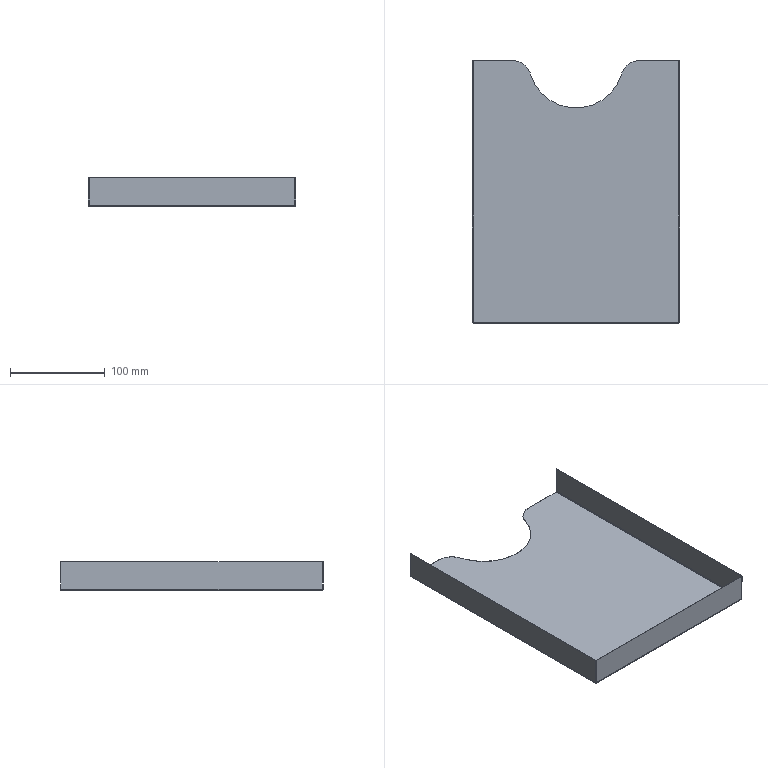Part | SolidWorks | features MirrorStock 1 | 1 solid | 34 faces | box 219 x 277 x 30 mm | volume 39482 mm3 | plane 21 | cylinder 9 | spline 4 | commonest cylinder face diameters 1.473 x3 2.473 x3 40 x2 100 x1
STEP:
#1=CARTESIAN_POINT('',(-67.082,138.5,0.));
#2=VERTEX_POINT('',#1);
#3=CARTESIAN_POINT('',(-108.263,138.5,0.));
#4=VERTEX_POINT('',#3);
#5=CARTESIAN_POINT('',(-109.5,138.5,0.));
#6=DIRECTION('',(-1.,0.,0.));
#7=VECTOR('',#6,1000.);
#8=LINE('',#5,#7);
#9=EDGE_CURVE('',#2,#4,#8,.T.);
#10=ORIENTED_EDGE('',*,*,#9,.T.);
#11=CARTESIAN_POINT('',(-108.263,138.5,0.5));
#12=VERTEX_POINT('',#11);
#13=CARTESIAN_POINT('',(-108.263,138.5,0.5));
#14=DIRECTION('',(0.,0.,-1.));
#15=VECTOR('',#14,1000.);
#16=LINE('',#13,#15);
#17=EDGE_CURVE('',#12,#4,#16,.T.);
#18=ORIENTED_EDGE('',*,*,#17,.F.);
#19=CARTESIAN_POINT('',(-67.082,138.5,0.5));
#20=VERTEX_POINT('',#19);
#21=CARTESIAN_POINT('',(-109.5,138.5,0.5));
#22=DIRECTION('',(-1.,0.,0.));
#23=VECTOR('',#22,1000.);
#24=LINE('',#21,#23);
#25=EDGE_CURVE('',#20,#12,#24,.T.);
#26=ORIENTED_EDGE('',*,*,#25,.F.);
#27=CARTESIAN_POINT('',(-67.082,138.5,0.5));
#28=DIRECTION('',(0.,0.,1.));
#29=VECTOR('',#28,1000.);
#30=LINE('',#27,#29);
#31=EDGE_CURVE('',#2,#20,#30,.T.);
#32=ORIENTED_EDGE('',*,*,#31,.F.);
#33=EDGE_LOOP('',(#10,#18,#26,#32));
#34=FACE_OUTER_BOUND('',#33,.T.);
#35=CARTESIAN_POINT('',(-109.5,138.5,0.5));
#36=DIRECTION('',(0.,1.,0.));
#37=DIRECTION('',(0.,0.,-1.));
#38=AXIS2_PLACEMENT_3D('',#35,#36,#37);
#39=PLANE('',#38);
#40=ADVANCED_FACE('',(#34),#39,.T.);
#41=CARTESIAN_POINT('',(-47.916,124.214,0.5));
#42=VERTEX_POINT('',#41);
#43=CARTESIAN_POINT('',(47.916,124.214,0.5));
#44=VERTEX_POINT('',#43);
#45=CARTESIAN_POINT('',(0.,138.5,0.5));
#46=DIRECTION('',(0.,0.,1.));
#47=DIRECTION('',(0.,-1.,0.));
#48=AXIS2_PLACEMENT_3D('',#45,#46,#47);
#49=CIRCLE('',#48,50.);
#50=EDGE_CURVE('',#42,#44,#49,.T.);
#51=ORIENTED_EDGE('',*,*,#50,.F.);
#52=CARTESIAN_POINT('',(-67.082,118.5,0.5));
#53=DIRECTION('',(0.,0.,-1.));
#54=DIRECTION('',(0.,-1.,0.));
#55=AXIS2_PLACEMENT_3D('',#52,#53,#54);
#56=CIRCLE('',#55,20.);
#57=EDGE_CURVE('',#20,#42,#56,.T.);
#58=ORIENTED_EDGE('',*,*,#57,.F.);
#59=ORIENTED_EDGE('',*,*,#25,.T.);
#60=CARTESIAN_POINT('',(-108.263,-137.263,0.5));
#61=VERTEX_POINT('',#60);
#62=CARTESIAN_POINT('',(-108.263,138.5,0.5));
#63=DIRECTION('',(0.,-1.,0.));
#64=VECTOR('',#63,1000.);
#65=LINE('',#62,#64);
#66=EDGE_CURVE('',#12,#61,#65,.T.);
#67=ORIENTED_EDGE('',*,*,#66,.T.);
#68=CARTESIAN_POINT('',(108.263,-137.263,0.5));
#69=VERTEX_POINT('',#68);
#70=CARTESIAN_POINT('',(-108.293,-137.263,0.5));
#71=DIRECTION('',(1.,0.,0.));
#72=VECTOR('',#71,1000.);
#73=LINE('',#70,#72);
#74=EDGE_CURVE('',#61,#69,#73,.T.);
#75=ORIENTED_EDGE('',*,*,#74,.T.);
#76=CARTESIAN_POINT('',(108.263,138.5,0.5));
#77=VERTEX_POINT('',#76);
#78=CARTESIAN_POINT('',(108.263,-137.293,0.5));
#79=DIRECTION('',(0.,1.,0.));
#80=VECTOR('',#79,1000.);
#81=LINE('',#78,#80);
#82=EDGE_CURVE('',#69,#77,#81,.T.);
#83=ORIENTED_EDGE('',*,*,#82,.T.);
#84=CARTESIAN_POINT('',(67.082,138.5,0.5));
#85=VERTEX_POINT('',#84);
#86=CARTESIAN_POINT('',(-109.5,138.5,0.5));
#87=DIRECTION('',(-1.,0.,0.));
#88=VECTOR('',#87,1000.);
#89=LINE('',#86,#88);
#90=EDGE_CURVE('',#77,#85,#89,.T.);
#91=ORIENTED_EDGE('',*,*,#90,.T.);
#92=CARTESIAN_POINT('',(67.082,118.5,0.5));
#93=DIRECTION('',(0.,0.,-1.));
#94=DIRECTION('',(0.,-1.,0.));
#95=AXIS2_PLACEMENT_3D('',#92,#93,#94);
#96=CIRCLE('',#95,20.);
#97=EDGE_CURVE('',#44,#85,#96,.T.);
#98=ORIENTED_EDGE('',*,*,#97,.F.);
#99=EDGE_LOOP('',(#51,#58,#59,#67,#75,#83,#91,#98));
#100=FACE_OUTER_BOUND('',#99,.T.);
#101=CARTESIAN_POINT('',(0.,0.,0.5));
#102=DIRECTION('',(0.,0.,-1.));
#103=DIRECTION('',(1.,0.,0.));
#104=AXIS2_PLACEMENT_3D('',#101,#102,#103);
#105=PLANE('',#104);
#106=ADVANCED_FACE('',(#100),#105,.F.);
#107=CARTESIAN_POINT('',(108.263,138.5,0.));
#108=VERTEX_POINT('',#107);
#109=CARTESIAN_POINT('',(67.082,138.5,0.));
#110=VERTEX_POINT('',#109);
#111=CARTESIAN_POINT('',(-109.5,138.5,0.));
#112=DIRECTION('',(-1.,0.,0.));
#113=VECTOR('',#112,1000.);
#114=LINE('',#111,#113);
#115=EDGE_CURVE('',#108,#110,#114,.T.);
#116=ORIENTED_EDGE('',*,*,#115,.F.);
#117=CARTESIAN_POINT('',(108.263,-137.263,0.));
#118=VERTEX_POINT('',#117);
#119=CARTESIAN_POINT('',(108.263,-137.293,0.));
#120=DIRECTION('',(0.,1.,0.));
#121=VECTOR('',#120,1000.);
#122=LINE('',#119,#121);
#123=EDGE_CURVE('',#118,#108,#122,.T.);
#124=ORIENTED_EDGE('',*,*,#123,.F.);
#125=CARTESIAN_POINT('',(-108.263,-137.263,0.));
#126=VERTEX_POINT('',#125);
#127=CARTESIAN_POINT('',(-108.293,-137.263,0.));
#128=DIRECTION('',(1.,0.,0.));
#129=VECTOR('',#128,1000.);
#130=LINE('',#127,#129);
#131=EDGE_CURVE('',#126,#118,#130,.T.);
#132=ORIENTED_EDGE('',*,*,#131,.F.);
#133=CARTESIAN_POINT('',(-108.263,138.5,0.));
#134=DIRECTION('',(0.,-1.,0.));
#135=VECTOR('',#134,1000.);
#136=LINE('',#133,#135);
#137=EDGE_CURVE('',#4,#126,#136,.T.);
#138=ORIENTED_EDGE('',*,*,#137,.F.);
#139=ORIENTED_EDGE('',*,*,#9,.F.);
#140=CARTESIAN_POINT('',(-47.916,124.214,0.));
#141=VERTEX_POINT('',#140);
#142=CARTESIAN_POINT('',(-67.082,118.5,0.));
#143=DIRECTION('',(0.,0.,1.));
#144=DIRECTION('',(0.,-1.,0.));
#145=AXIS2_PLACEMENT_3D('',#142,#143,#144);
#146=CIRCLE('',#145,20.);
#147=EDGE_CURVE('',#141,#2,#146,.T.);
#148=ORIENTED_EDGE('',*,*,#147,.F.);
#149=CARTESIAN_POINT('',(47.916,124.214,0.));
#150=VERTEX_POINT('',#149);
#151=CARTESIAN_POINT('',(0.,138.5,0.));
#152=DIRECTION('',(0.,0.,1.));
#153=DIRECTION('',(1.,0.,0.));
#154=AXIS2_PLACEMENT_3D('',#151,#152,#153);
#155=CIRCLE('',#154,50.);
#156=EDGE_CURVE('',#141,#150,#155,.T.);
#157=ORIENTED_EDGE('',*,*,#156,.T.);
#158=CARTESIAN_POINT('',(67.082,118.5,0.));
#159=DIRECTION('',(0.,0.,1.));
#160=DIRECTION('',(0.,-1.,0.));
#161=AXIS2_PLACEMENT_3D('',#158,#159,#160);
#162=CIRCLE('',#161,20.);
#163=EDGE_CURVE('',#110,#150,#162,.T.);
#164=ORIENTED_EDGE('',*,*,#163,.F.);
#165=EDGE_LOOP('',(#116,#124,#132,#138,#139,#148,#157,#164));
#166=FACE_OUTER_BOUND('',#165,.T.);
#167=CARTESIAN_POINT('',(0.,0.,0.));
#168=DIRECTION('',(0.,0.,-1.));
#169=DIRECTION('',(1.,0.,0.));
#170=AXIS2_PLACEMENT_3D('',#167,#168,#169);
#171=PLANE('',#170);
#172=ADVANCED_FACE('',(#166),#171,.T.);
#173=ORIENTED_EDGE('',*,*,#90,.F.);
#174=CARTESIAN_POINT('',(108.263,138.5,0.5));
#175=DIRECTION('',(0.,0.,-1.));
#176=VECTOR('',#175,1000.);
#177=LINE('',#174,#176);
#178=EDGE_CURVE('',#77,#108,#177,.T.);
#179=ORIENTED_EDGE('',*,*,#178,.T.);
#180=ORIENTED_EDGE('',*,*,#115,.T.);
#181=CARTESIAN_POINT('',(67.082,138.5,0.));
#182=DIRECTION('',(0.,0.,-1.));
#183=VECTOR('',#182,1000.);
#184=LINE('',#181,#183);
#185=EDGE_CURVE('',#85,#110,#184,.T.);
#186=ORIENTED_EDGE('',*,*,#185,.F.);
#187=EDGE_LOOP('',(#173,#179,#180,#186));
#188=FACE_OUTER_BOUND('',#187,.T.);
#189=CARTESIAN_POINT('',(-109.5,138.5,0.5));
#190=DIRECTION('',(0.,1.,0.));
#191=DIRECTION('',(0.,0.,-1.));
#192=AXIS2_PLACEMENT_3D('',#189,#190,#191);
#193=PLANE('',#192);
#194=ADVANCED_FACE('',(#188),#193,.T.);
#195=CARTESIAN_POINT('',(-109.5,-137.293,1.237));
#196=VERTEX_POINT('',#195);
#197=CARTESIAN_POINT('',(-109.,-137.293,1.237));
#198=VERTEX_POINT('',#197);
#199=CARTESIAN_POINT('',(-109.,-137.293,1.237));
#200=DIRECTION('',(1.,0.,0.));
#201=VECTOR('',#200,1000.);
#202=LINE('',#199,#201);
#203=EDGE_CURVE('',#196,#198,#202,.T.);
#204=ORIENTED_EDGE('',*,*,#203,.F.);
#205=CARTESIAN_POINT('',(-108.263,-137.263,0.));
#206=CARTESIAN_POINT('',(-108.425,-137.266,0.));
#207=CARTESIAN_POINT('',(-108.587,-137.268,0.03219));
#208=CARTESIAN_POINT('',(-108.886,-137.273,0.1561));
#209=CARTESIAN_POINT('',(-109.023,-137.276,0.2477));
#210=CARTESIAN_POINT('',(-109.252,-137.281,0.4767));
#211=CARTESIAN_POINT('',(-109.344,-137.283,0.6138));
#212=CARTESIAN_POINT('',(-109.468,-137.288,0.9129));
#213=CARTESIAN_POINT('',(-109.5,-137.29,1.075));
#214=CARTESIAN_POINT('',(-109.5,-137.293,1.237));
#215=B_SPLINE_CURVE_WITH_KNOTS('',3,(#205,#206,#207,#208,#209,#210,#211,#212,#213,#214),.UNSPECIFIED.,.F.,.F.,(4,2,2,2,4),(0.,0.25,0.5,0.75,1.),.UNSPECIFIED.);
#216=EDGE_CURVE('',#126,#196,#215,.T.);
#217=ORIENTED_EDGE('',*,*,#216,.F.);
#218=CARTESIAN_POINT('',(-108.263,-137.263,0.5));
#219=DIRECTION('',(0.,0.,-1.));
#220=VECTOR('',#219,1000.);
#221=LINE('',#218,#220);
#222=EDGE_CURVE('',#61,#126,#221,.T.);
#223=ORIENTED_EDGE('',*,*,#222,.F.);
#224=CARTESIAN_POINT('',(-108.263,-137.263,0.5));
#225=CARTESIAN_POINT('',(-108.456,-137.268,0.5));
#226=CARTESIAN_POINT('',(-108.648,-137.273,0.5794));
#227=CARTESIAN_POINT('',(-108.921,-137.283,0.8521));
#228=CARTESIAN_POINT('',(-109.,-137.288,1.044));
#229=CARTESIAN_POINT('',(-109.,-137.293,1.237));
#230=B_SPLINE_CURVE_WITH_KNOTS('',3,(#224,#225,#226,#227,#228,#229),.UNSPECIFIED.,.F.,.F.,(4,2,4),(0.,0.5,1.),.UNSPECIFIED.);
#231=EDGE_CURVE('',#61,#198,#230,.T.);
#232=ORIENTED_EDGE('',*,*,#231,.T.);
#233=EDGE_LOOP('',(#204,#217,#223,#232));
#234=FACE_OUTER_BOUND('',#233,.T.);
#235=CARTESIAN_POINT('',(-108.263,-137.263,-0.005));
#236=CARTESIAN_POINT('',(-108.426,-137.266,-0.005));
#237=CARTESIAN_POINT('',(-108.588,-137.268,0.02732));
#238=CARTESIAN_POINT('',(-108.889,-137.273,0.1517));
#239=CARTESIAN_POINT('',(-109.026,-137.276,0.2437));
#240=CARTESIAN_POINT('',(-109.256,-137.281,0.4736));
#241=CARTESIAN_POINT('',(-109.348,-137.283,0.6113));
#242=CARTESIAN_POINT('',(-109.473,-137.288,0.9116));
#243=CARTESIAN_POINT('',(-109.505,-137.29,1.074));
#244=CARTESIAN_POINT('',(-109.505,-137.293,1.237));
#245=CARTESIAN_POINT('',(-108.263,-137.263,0.));
#246=CARTESIAN_POINT('',(-108.425,-137.266,0.));
#247=CARTESIAN_POINT('',(-108.587,-137.268,0.03219));
#248=CARTESIAN_POINT('',(-108.886,-137.273,0.1561));
#249=CARTESIAN_POINT('',(-109.023,-137.276,0.2477));
#250=CARTESIAN_POINT('',(-109.252,-137.281,0.4767));
#251=CARTESIAN_POINT('',(-109.344,-137.283,0.6138));
#252=CARTESIAN_POINT('',(-109.468,-137.288,0.9129));
#253=CARTESIAN_POINT('',(-109.5,-137.29,1.075));
#254=CARTESIAN_POINT('',(-109.5,-137.293,1.237));
#255=CARTESIAN_POINT('',(-108.263,-137.263,0.5));
#256=CARTESIAN_POINT('',(-108.36,-137.266,0.5));
#257=CARTESIAN_POINT('',(-108.456,-137.268,0.5192));
#258=CARTESIAN_POINT('',(-108.634,-137.273,0.593));
#259=CARTESIAN_POINT('',(-108.716,-137.276,0.6476));
#260=CARTESIAN_POINT('',(-108.852,-137.281,0.7839));
#261=CARTESIAN_POINT('',(-108.907,-137.283,0.8656));
#262=CARTESIAN_POINT('',(-108.981,-137.288,1.044));
#263=CARTESIAN_POINT('',(-109.,-137.29,1.14));
#264=CARTESIAN_POINT('',(-109.,-137.293,1.237));
#265=CARTESIAN_POINT('',(-108.263,-137.263,0.5051));
#266=CARTESIAN_POINT('',(-108.359,-137.266,0.5051));
#267=CARTESIAN_POINT('',(-108.455,-137.268,0.5241));
#268=CARTESIAN_POINT('',(-108.632,-137.273,0.5974));
#269=CARTESIAN_POINT('',(-108.713,-137.276,0.6516));
#270=CARTESIAN_POINT('',(-108.848,-137.281,0.787));
#271=CARTESIAN_POINT('',(-108.903,-137.283,0.8682));
#272=CARTESIAN_POINT('',(-108.976,-137.288,1.045));
#273=CARTESIAN_POINT('',(-108.995,-137.29,1.141));
#274=CARTESIAN_POINT('',(-108.995,-137.293,1.237));
#275=B_SPLINE_SURFACE_WITH_KNOTS('',1,3,((#235,#236,#237,#238,#239,#240,#241,#242,#243,#244),(#245,#246,#247,#248,#249,#250,#251,#252,#253,#254),(#255,#256,#257,#258,#259,#260,#261,#262,#263,#264),(#265,#266,#267,#268,#269,#270,#271,#272,#273,#274)),.UNSPECIFIED.,.F.,.F.,.F.,(2,1,1,2),(4,2,2,2,4),(-0.01,0.,1.,1.01),(0.,0.25,0.5,0.75,1.),.UNSPECIFIED.);
#276=ADVANCED_FACE('',(#234),#275,.T.);
#277=CARTESIAN_POINT('',(-109.,138.5,1.237));
#278=VERTEX_POINT('',#277);
#279=CARTESIAN_POINT('',(-108.263,138.5,1.237));
#280=DIRECTION('',(0.,-1.,0.));
#281=DIRECTION('',(0.,0.,-1.));
#282=AXIS2_PLACEMENT_3D('',#279,#280,#281);
#283=CIRCLE('',#282,0.7366);
#284=EDGE_CURVE('',#278,#12,#283,.T.);
#285=ORIENTED_EDGE('',*,*,#284,.T.);
#286=ORIENTED_EDGE('',*,*,#17,.T.);
#287=CARTESIAN_POINT('',(-109.5,138.5,1.237));
#288=VERTEX_POINT('',#287);
#289=CARTESIAN_POINT('',(-108.263,138.5,1.237));
#290=DIRECTION('',(0.,-1.,0.));
#291=DIRECTION('',(0.,0.,-1.));
#292=AXIS2_PLACEMENT_3D('',#289,#290,#291);
#293=CIRCLE('',#292,1.237);
#294=EDGE_CURVE('',#288,#4,#293,.T.);
#295=ORIENTED_EDGE('',*,*,#294,.F.);
#296=CARTESIAN_POINT('',(-109.,138.5,1.237));
#297=DIRECTION('',(-1.,0.,0.));
#298=VECTOR('',#297,1000.);
#299=LINE('',#296,#298);
#300=EDGE_CURVE('',#278,#288,#299,.T.);
#301=ORIENTED_EDGE('',*,*,#300,.F.);
#302=EDGE_LOOP('',(#285,#286,#295,#301));
#303=FACE_OUTER_BOUND('',#302,.T.);
#304=CARTESIAN_POINT('',(-108.263,138.5,1.237));
#305=DIRECTION('',(0.,-1.,0.));
#306=DIRECTION('',(0.,0.,1.));
#307=AXIS2_PLACEMENT_3D('',#304,#305,#306);
#308=PLANE('',#307);
#309=ADVANCED_FACE('',(#303),#308,.F.);
#310=ORIENTED_EDGE('',*,*,#137,.T.);
#311=ORIENTED_EDGE('',*,*,#216,.T.);
#312=CARTESIAN_POINT('',(-109.5,0.,1.237));
#313=DIRECTION('',(0.,1.,0.));
#314=VECTOR('',#313,1000.);
#315=LINE('',#312,#314);
#316=EDGE_CURVE('',#196,#288,#315,.T.);
#317=ORIENTED_EDGE('',*,*,#316,.T.);
#318=ORIENTED_EDGE('',*,*,#294,.T.);
#319=EDGE_LOOP('',(#310,#311,#317,#318));
#320=FACE_OUTER_BOUND('',#319,.T.);
#321=CARTESIAN_POINT('',(-108.263,138.5,1.237));
#322=DIRECTION('',(0.,1.,0.));
#323=DIRECTION('',(-1.,0.,0.));
#324=AXIS2_PLACEMENT_3D('',#321,#322,#323);
#325=CYLINDRICAL_SURFACE('',#324,1.237);
#326=ADVANCED_FACE('',(#320),#325,.T.);
#327=ORIENTED_EDGE('',*,*,#66,.F.);
#328=ORIENTED_EDGE('',*,*,#284,.F.);
#329=CARTESIAN_POINT('',(-109.,-138.5,1.237));
#330=DIRECTION('',(0.,1.,0.));
#331=VECTOR('',#330,1000.);
#332=LINE('',#329,#331);
#333=EDGE_CURVE('',#198,#278,#332,.T.);
#334=ORIENTED_EDGE('',*,*,#333,.F.);
#335=ORIENTED_EDGE('',*,*,#231,.F.);
#336=EDGE_LOOP('',(#327,#328,#334,#335));
#337=FACE_OUTER_BOUND('',#336,.T.);
#338=CARTESIAN_POINT('',(-108.263,138.5,1.237));
#339=DIRECTION('',(0.,1.,0.));
#340=DIRECTION('',(-1.,0.,0.));
#341=AXIS2_PLACEMENT_3D('',#338,#339,#340);
#342=CYLINDRICAL_SURFACE('',#341,0.7366);
#343=ADVANCED_FACE('',(#337),#342,.F.);
#344=CARTESIAN_POINT('',(-109.,-137.293,30.));
#345=VERTEX_POINT('',#344);
#346=CARTESIAN_POINT('',(-109.5,-137.293,30.));
#347=VERTEX_POINT('',#346);
#348=CARTESIAN_POINT('',(-109.5,-137.293,30.));
#349=DIRECTION('',(-1.,0.,0.));
#350=VECTOR('',#349,1000.);
#351=LINE('',#348,#350);
#352=EDGE_CURVE('',#345,#347,#351,.T.);
#353=ORIENTED_EDGE('',*,*,#352,.T.);
#354=CARTESIAN_POINT('',(-109.5,-137.293,0.));
#355=DIRECTION('',(0.,0.,-1.));
#356=VECTOR('',#355,1000.);
#357=LINE('',#354,#356);
#358=EDGE_CURVE('',#347,#196,#357,.T.);
#359=ORIENTED_EDGE('',*,*,#358,.T.);
#360=ORIENTED_EDGE('',*,*,#203,.T.);
#361=CARTESIAN_POINT('',(-109.,-137.293,0.));
#362=DIRECTION('',(0.,0.,1.));
#363=VECTOR('',#362,1000.);
#364=LINE('',#361,#363);
#365=EDGE_CURVE('',#198,#345,#364,.T.);
#366=ORIENTED_EDGE('',*,*,#365,.T.);
#367=EDGE_LOOP('',(#353,#359,#360,#366));
#368=FACE_OUTER_BOUND('',#367,.T.);
#369=CARTESIAN_POINT('',(-109.,-137.293,0.5));
#370=DIRECTION('',(0.,-1.,0.));
#371=DIRECTION('',(0.,0.,1.));
#372=AXIS2_PLACEMENT_3D('',#369,#370,#371);
#373=PLANE('',#372);
#374=ADVANCED_FACE('',(#368),#373,.T.);
#375=CARTESIAN_POINT('',(-109.5,138.5,30.));
#376=VERTEX_POINT('',#375);
#377=CARTESIAN_POINT('',(-109.5,138.5,30.));
#378=DIRECTION('',(0.,1.,0.));
#379=VECTOR('',#378,1000.);
#380=LINE('',#377,#379);
#381=EDGE_CURVE('',#347,#376,#380,.T.);
#382=ORIENTED_EDGE('',*,*,#381,.T.);
#383=CARTESIAN_POINT('',(-109.5,138.5,0.5));
#384=DIRECTION('',(0.,0.,-1.));
#385=VECTOR('',#384,1000.);
#386=LINE('',#383,#385);
#387=EDGE_CURVE('',#376,#288,#386,.T.);
#388=ORIENTED_EDGE('',*,*,#387,.T.);
#389=ORIENTED_EDGE('',*,*,#316,.F.);
#390=ORIENTED_EDGE('',*,*,#358,.F.);
#391=EDGE_LOOP('',(#382,#388,#389,#390));
#392=FACE_OUTER_BOUND('',#391,.T.);
#393=CARTESIAN_POINT('',(-109.5,0.,0.));
#394=DIRECTION('',(-1.,0.,0.));
#395=DIRECTION('',(0.,0.,-1.));
#396=AXIS2_PLACEMENT_3D('',#393,#394,#395);
#397=PLANE('',#396);
#398=ADVANCED_FACE('',(#392),#397,.T.);
#399=ORIENTED_EDGE('',*,*,#365,.F.);
#400=ORIENTED_EDGE('',*,*,#333,.T.);
#401=CARTESIAN_POINT('',(-109.,138.5,30.));
#402=VERTEX_POINT('',#401);
#403=CARTESIAN_POINT('',(-109.,138.5,0.));
#404=DIRECTION('',(0.,0.,-1.));
#405=VECTOR('',#404,1000.);
#406=LINE('',#403,#405);
#407=EDGE_CURVE('',#402,#278,#406,.T.);
#408=ORIENTED_EDGE('',*,*,#407,.F.);
#409=CARTESIAN_POINT('',(-109.,0.,30.));
#410=DIRECTION('',(0.,1.,0.));
#411=VECTOR('',#410,1000.);
#412=LINE('',#409,#411);
#413=EDGE_CURVE('',#345,#402,#412,.T.);
#414=ORIENTED_EDGE('',*,*,#413,.F.);
#415=EDGE_LOOP('',(#399,#400,#408,#414));
#416=FACE_OUTER_BOUND('',#415,.T.);
#417=CARTESIAN_POINT('',(-109.,0.,0.));
#418=DIRECTION('',(-1.,0.,0.));
#419=DIRECTION('',(0.,0.,-1.));
#420=AXIS2_PLACEMENT_3D('',#417,#418,#419);
#421=PLANE('',#420);
#422=ADVANCED_FACE('',(#416),#421,.F.);
#423=ORIENTED_EDGE('',*,*,#413,.T.);
#424=CARTESIAN_POINT('',(-109.5,138.5,30.));
#425=DIRECTION('',(1.,0.,0.));
#426=VECTOR('',#425,1000.);
#427=LINE('',#424,#426);
#428=EDGE_CURVE('',#376,#402,#427,.T.);
#429=ORIENTED_EDGE('',*,*,#428,.F.);
#430=ORIENTED_EDGE('',*,*,#381,.F.);
#431=ORIENTED_EDGE('',*,*,#352,.F.);
#432=EDGE_LOOP('',(#423,#429,#430,#431));
#433=FACE_OUTER_BOUND('',#432,.T.);
#434=CARTESIAN_POINT('',(-109.5,138.5,30.));
#435=DIRECTION('',(0.,0.,1.));
#436=DIRECTION('',(-1.,0.,0.));
#437=AXIS2_PLACEMENT_3D('',#434,#435,#436);
#438=PLANE('',#437);
#439=ADVANCED_FACE('',(#433),#438,.T.);
#440=ORIENTED_EDGE('',*,*,#387,.F.);
#441=ORIENTED_EDGE('',*,*,#428,.T.);
#442=ORIENTED_EDGE('',*,*,#407,.T.);
#443=ORIENTED_EDGE('',*,*,#300,.T.);
#444=EDGE_LOOP('',(#440,#441,#442,#443));
#445=FACE_OUTER_BOUND('',#444,.T.);
#446=CARTESIAN_POINT('',(-109.5,138.5,0.5));
#447=DIRECTION('',(0.,1.,0.));
#448=DIRECTION('',(0.,0.,-1.));
#449=AXIS2_PLACEMENT_3D('',#446,#447,#448);
#450=PLANE('',#449);
#451=ADVANCED_FACE('',(#445),#450,.T.);
#452=CARTESIAN_POINT('',(109.,138.5,1.237));
#453=VERTEX_POINT('',#452);
#454=CARTESIAN_POINT('',(109.5,138.5,1.237));
#455=VERTEX_POINT('',#454);
#456=CARTESIAN_POINT('',(109.5,138.5,1.237));
#457=DIRECTION('',(1.,0.,0.));
#458=VECTOR('',#457,1000.);
#459=LINE('',#456,#458);
#460=EDGE_CURVE('',#453,#455,#459,.T.);
#461=ORIENTED_EDGE('',*,*,#460,.T.);
#462=CARTESIAN_POINT('',(108.263,138.5,1.237));
#463=DIRECTION('',(0.,-1.,0.));
#464=DIRECTION('',(0.,0.,1.));
#465=AXIS2_PLACEMENT_3D('',#462,#463,#464);
#466=CIRCLE('',#465,1.237);
#467=EDGE_CURVE('',#108,#455,#466,.T.);
#468=ORIENTED_EDGE('',*,*,#467,.F.);
#469=ORIENTED_EDGE('',*,*,#178,.F.);
#470=CARTESIAN_POINT('',(108.263,138.5,1.237));
#471=DIRECTION('',(0.,-1.,0.));
#472=DIRECTION('',(0.,0.,1.));
#473=AXIS2_PLACEMENT_3D('',#470,#471,#472);
#474=CIRCLE('',#473,0.7366);
#475=EDGE_CURVE('',#77,#453,#474,.T.);
#476=ORIENTED_EDGE('',*,*,#475,.T.);
#477=EDGE_LOOP('',(#461,#468,#469,#476));
#478=FACE_OUTER_BOUND('',#477,.T.);
#479=CARTESIAN_POINT('',(108.263,138.5,1.237));
#480=DIRECTION('',(0.,1.,0.));
#481=DIRECTION('',(0.,0.,-1.));
#482=AXIS2_PLACEMENT_3D('',#479,#480,#481);
#483=PLANE('',#482);
#484=ADVANCED_FACE('',(#478),#483,.T.);
#485=CARTESIAN_POINT('',(109.,-137.293,1.237));
#486=VERTEX_POINT('',#485);
#487=CARTESIAN_POINT('',(109.,-137.293,1.237));
#488=CARTESIAN_POINT('',(109.,-137.288,1.044));
#489=CARTESIAN_POINT('',(108.921,-137.283,0.8521));
#490=CARTESIAN_POINT('',(108.648,-137.273,0.5794));
#491=CARTESIAN_POINT('',(108.456,-137.268,0.5));
#492=CARTESIAN_POINT('',(108.263,-137.263,0.5));
#493=B_SPLINE_CURVE_WITH_KNOTS('',3,(#487,#488,#489,#490,#491,#492),.UNSPECIFIED.,.F.,.F.,(4,2,4),(0.,0.5,1.),.UNSPECIFIED.);
#494=EDGE_CURVE('',#486,#69,#493,.T.);
#495=ORIENTED_EDGE('',*,*,#494,.T.);
#496=CARTESIAN_POINT('',(108.263,-137.263,0.5));
#497=DIRECTION('',(0.,0.,-1.));
#498=VECTOR('',#497,1000.);
#499=LINE('',#496,#498);
#500=EDGE_CURVE('',#69,#118,#499,.T.);
#501=ORIENTED_EDGE('',*,*,#500,.T.);
#502=CARTESIAN_POINT('',(109.5,-137.293,1.237));
#503=VERTEX_POINT('',#502);
#504=CARTESIAN_POINT('',(109.5,-137.293,1.237));
#505=CARTESIAN_POINT('',(109.5,-137.29,1.075));
#506=CARTESIAN_POINT('',(109.468,-137.288,0.9129));
#507=CARTESIAN_POINT('',(109.344,-137.283,0.6138));
#508=CARTESIAN_POINT('',(109.252,-137.281,0.4767));
#509=CARTESIAN_POINT('',(109.023,-137.276,0.2477));
#510=CARTESIAN_POINT('',(108.886,-137.273,0.1561));
#511=CARTESIAN_POINT('',(108.587,-137.268,0.03219));
#512=CARTESIAN_POINT('',(108.425,-137.266,0.));
#513=CARTESIAN_POINT('',(108.263,-137.263,0.));
#514=B_SPLINE_CURVE_WITH_KNOTS('',3,(#504,#505,#506,#507,#508,#509,#510,#511,#512,#513),.UNSPECIFIED.,.F.,.F.,(4,2,2,2,4),(0.,0.25,0.5,0.75,1.),.UNSPECIFIED.);
#515=EDGE_CURVE('',#503,#118,#514,.T.);
#516=ORIENTED_EDGE('',*,*,#515,.F.);
#517=CARTESIAN_POINT('',(109.,-137.293,1.237));
#518=DIRECTION('',(-1.,0.,0.));
#519=VECTOR('',#518,1000.);
#520=LINE('',#517,#519);
#521=EDGE_CURVE('',#503,#486,#520,.T.);
#522=ORIENTED_EDGE('',*,*,#521,.T.);
#523=EDGE_LOOP('',(#495,#501,#516,#522));
#524=FACE_OUTER_BOUND('',#523,.T.);
#525=CARTESIAN_POINT('',(109.505,-137.293,1.237));
#526=CARTESIAN_POINT('',(109.505,-137.29,1.074));
#527=CARTESIAN_POINT('',(109.473,-137.288,0.9116));
#528=CARTESIAN_POINT('',(109.348,-137.283,0.6113));
#529=CARTESIAN_POINT('',(109.256,-137.281,0.4736));
#530=CARTESIAN_POINT('',(109.026,-137.276,0.2437));
#531=CARTESIAN_POINT('',(108.889,-137.273,0.1517));
#532=CARTESIAN_POINT('',(108.588,-137.268,0.02732));
#533=CARTESIAN_POINT('',(108.426,-137.266,-0.005));
#534=CARTESIAN_POINT('',(108.263,-137.263,-0.005));
#535=CARTESIAN_POINT('',(109.5,-137.293,1.237));
#536=CARTESIAN_POINT('',(109.5,-137.29,1.075));
#537=CARTESIAN_POINT('',(109.468,-137.288,0.9129));
#538=CARTESIAN_POINT('',(109.344,-137.283,0.6138));
#539=CARTESIAN_POINT('',(109.252,-137.281,0.4767));
#540=CARTESIAN_POINT('',(109.023,-137.276,0.2477));
#541=CARTESIAN_POINT('',(108.886,-137.273,0.1561));
#542=CARTESIAN_POINT('',(108.587,-137.268,0.03219));
#543=CARTESIAN_POINT('',(108.425,-137.266,0.));
#544=CARTESIAN_POINT('',(108.263,-137.263,0.));
#545=CARTESIAN_POINT('',(109.,-137.293,1.237));
#546=CARTESIAN_POINT('',(109.,-137.29,1.14));
#547=CARTESIAN_POINT('',(108.981,-137.288,1.044));
#548=CARTESIAN_POINT('',(108.907,-137.283,0.8656));
#549=CARTESIAN_POINT('',(108.852,-137.281,0.7839));
#550=CARTESIAN_POINT('',(108.716,-137.276,0.6476));
#551=CARTESIAN_POINT('',(108.634,-137.273,0.593));
#552=CARTESIAN_POINT('',(108.456,-137.268,0.5192));
#553=CARTESIAN_POINT('',(108.36,-137.266,0.5));
#554=CARTESIAN_POINT('',(108.263,-137.263,0.5));
#555=CARTESIAN_POINT('',(108.995,-137.293,1.237));
#556=CARTESIAN_POINT('',(108.995,-137.29,1.141));
#557=CARTESIAN_POINT('',(108.976,-137.288,1.045));
#558=CARTESIAN_POINT('',(108.903,-137.283,0.8682));
#559=CARTESIAN_POINT('',(108.848,-137.281,0.787));
#560=CARTESIAN_POINT('',(108.713,-137.276,0.6516));
#561=CARTESIAN_POINT('',(108.632,-137.273,0.5974));
#562=CARTESIAN_POINT('',(108.455,-137.268,0.5241));
#563=CARTESIAN_POINT('',(108.359,-137.266,0.505));
#564=CARTESIAN_POINT('',(108.263,-137.263,0.505));
#565=B_SPLINE_SURFACE_WITH_KNOTS('',1,3,((#525,#526,#527,#528,#529,#530,#531,#532,#533,#534),(#535,#536,#537,#538,#539,#540,#541,#542,#543,#544),(#545,#546,#547,#548,#549,#550,#551,#552,#553,#554),(#555,#556,#557,#558,#559,#560,#561,#562,#563,#564)),.UNSPECIFIED.,.F.,.F.,.F.,(2,1,1,2),(4,2,2,2,4),(-0.01,0.,1.,1.01),(0.,0.25,0.5,0.75,1.),.UNSPECIFIED.);
#566=ADVANCED_FACE('',(#524),#565,.T.);
#567=ORIENTED_EDGE('',*,*,#123,.T.);
#568=ORIENTED_EDGE('',*,*,#467,.T.);
#569=CARTESIAN_POINT('',(109.5,138.5,1.237));
#570=DIRECTION('',(0.,1.,0.));
#571=VECTOR('',#570,1000.);
#572=LINE('',#569,#571);
#573=EDGE_CURVE('',#503,#455,#572,.T.);
#574=ORIENTED_EDGE('',*,*,#573,.F.);
#575=ORIENTED_EDGE('',*,*,#515,.T.);
#576=EDGE_LOOP('',(#567,#568,#574,#575));
#577=FACE_OUTER_BOUND('',#576,.T.);
#578=CARTESIAN_POINT('',(108.263,-137.293,1.237));
#579=DIRECTION('',(0.,-1.,0.));
#580=DIRECTION('',(1.,0.,0.));
#581=AXIS2_PLACEMENT_3D('',#578,#579,#580);
#582=CYLINDRICAL_SURFACE('',#581,1.237);
#583=ADVANCED_FACE('',(#577),#582,.T.);
#584=ORIENTED_EDGE('',*,*,#82,.F.);
#585=ORIENTED_EDGE('',*,*,#494,.F.);
#586=CARTESIAN_POINT('',(109.,138.5,1.237));
#587=DIRECTION('',(0.,-1.,0.));
#588=VECTOR('',#587,1000.);
#589=LINE('',#586,#588);
#590=EDGE_CURVE('',#453,#486,#589,.T.);
#591=ORIENTED_EDGE('',*,*,#590,.F.);
#592=ORIENTED_EDGE('',*,*,#475,.F.);
#593=EDGE_LOOP('',(#584,#585,#591,#592));
#594=FACE_OUTER_BOUND('',#593,.T.);
#595=CARTESIAN_POINT('',(108.263,-137.293,1.237));
#596=DIRECTION('',(0.,-1.,0.));
#597=DIRECTION('',(1.,0.,0.));
#598=AXIS2_PLACEMENT_3D('',#595,#596,#597);
#599=CYLINDRICAL_SURFACE('',#598,0.7366);
#600=ADVANCED_FACE('',(#594),#599,.F.);
#601=CARTESIAN_POINT('',(109.,138.5,30.));
#602=VERTEX_POINT('',#601);
#603=CARTESIAN_POINT('',(109.,138.5,0.));
#604=DIRECTION('',(0.,0.,1.));
#605=VECTOR('',#604,1000.);
#606=LINE('',#603,#605);
#607=EDGE_CURVE('',#453,#602,#606,.T.);
#608=ORIENTED_EDGE('',*,*,#607,.T.);
#609=CARTESIAN_POINT('',(109.5,138.5,30.));
#610=VERTEX_POINT('',#609);
#611=CARTESIAN_POINT('',(109.5,138.5,30.));
#612=DIRECTION('',(-1.,0.,0.));
#613=VECTOR('',#612,1000.);
#614=LINE('',#611,#613);
#615=EDGE_CURVE('',#610,#602,#614,.T.);
#616=ORIENTED_EDGE('',*,*,#615,.F.);
#617=CARTESIAN_POINT('',(109.5,138.5,0.5));
#618=DIRECTION('',(0.,0.,1.));
#619=VECTOR('',#618,1000.);
#620=LINE('',#617,#619);
#621=EDGE_CURVE('',#455,#610,#620,.T.);
#622=ORIENTED_EDGE('',*,*,#621,.F.);
#623=ORIENTED_EDGE('',*,*,#460,.F.);
#624=EDGE_LOOP('',(#608,#616,#622,#623));
#625=FACE_OUTER_BOUND('',#624,.T.);
#626=CARTESIAN_POINT('',(109.5,138.5,0.5));
#627=DIRECTION('',(0.,1.,0.));
#628=DIRECTION('',(0.,0.,-1.));
#629=AXIS2_PLACEMENT_3D('',#626,#627,#628);
#630=PLANE('',#629);
#631=ADVANCED_FACE('',(#625),#630,.T.);
#632=ORIENTED_EDGE('',*,*,#573,.T.);
#633=ORIENTED_EDGE('',*,*,#621,.T.);
#634=CARTESIAN_POINT('',(109.5,-137.293,30.));
#635=VERTEX_POINT('',#634);
#636=CARTESIAN_POINT('',(109.5,138.5,30.));
#637=DIRECTION('',(0.,-1.,0.));
#638=VECTOR('',#637,1000.);
#639=LINE('',#636,#638);
#640=EDGE_CURVE('',#610,#635,#639,.T.);
#641=ORIENTED_EDGE('',*,*,#640,.T.);
#642=CARTESIAN_POINT('',(109.5,-137.293,0.));
#643=DIRECTION('',(0.,0.,1.));
#644=VECTOR('',#643,1000.);
#645=LINE('',#642,#644);
#646=EDGE_CURVE('',#503,#635,#645,.T.);
#647=ORIENTED_EDGE('',*,*,#646,.F.);
#648=EDGE_LOOP('',(#632,#633,#641,#647));
#649=FACE_OUTER_BOUND('',#648,.T.);
#650=CARTESIAN_POINT('',(109.5,0.,0.));
#651=DIRECTION('',(-1.,0.,0.));
#652=DIRECTION('',(0.,0.,-1.));
#653=AXIS2_PLACEMENT_3D('',#650,#651,#652);
#654=PLANE('',#653);
#655=ADVANCED_FACE('',(#649),#654,.F.);
#656=CARTESIAN_POINT('',(109.,-137.293,30.));
#657=VERTEX_POINT('',#656);
#658=CARTESIAN_POINT('',(109.,-137.293,0.5));
#659=DIRECTION('',(0.,0.,1.));
#660=VECTOR('',#659,1000.);
#661=LINE('',#658,#660);
#662=EDGE_CURVE('',#486,#657,#661,.T.);
#663=ORIENTED_EDGE('',*,*,#662,.T.);
#664=CARTESIAN_POINT('',(109.,0.,30.));
#665=DIRECTION('',(0.,-1.,0.));
#666=VECTOR('',#665,1000.);
#667=LINE('',#664,#666);
#668=EDGE_CURVE('',#602,#657,#667,.T.);
#669=ORIENTED_EDGE('',*,*,#668,.F.);
#670=ORIENTED_EDGE('',*,*,#607,.F.);
#671=ORIENTED_EDGE('',*,*,#590,.T.);
#672=EDGE_LOOP('',(#663,#669,#670,#671));
#673=FACE_OUTER_BOUND('',#672,.T.);
#674=CARTESIAN_POINT('',(109.,0.,0.));
#675=DIRECTION('',(-1.,0.,0.));
#676=DIRECTION('',(0.,0.,-1.));
#677=AXIS2_PLACEMENT_3D('',#674,#675,#676);
#678=PLANE('',#677);
#679=ADVANCED_FACE('',(#673),#678,.T.);
#680=CARTESIAN_POINT('',(109.,-137.293,30.));
#681=DIRECTION('',(1.,0.,0.));
#682=VECTOR('',#681,1000.);
#683=LINE('',#680,#682);
#684=EDGE_CURVE('',#657,#635,#683,.T.);
#685=ORIENTED_EDGE('',*,*,#684,.T.);
#686=ORIENTED_EDGE('',*,*,#640,.F.);
#687=ORIENTED_EDGE('',*,*,#615,.T.);
#688=ORIENTED_EDGE('',*,*,#668,.T.);
#689=EDGE_LOOP('',(#685,#686,#687,#688));
#690=FACE_OUTER_BOUND('',#689,.T.);
#691=CARTESIAN_POINT('',(109.5,138.5,30.));
#692=DIRECTION('',(0.,0.,1.));
#693=DIRECTION('',(-1.,0.,0.));
#694=AXIS2_PLACEMENT_3D('',#691,#692,#693);
#695=PLANE('',#694);
#696=ADVANCED_FACE('',(#690),#695,.T.);
#697=ORIENTED_EDGE('',*,*,#662,.F.);
#698=ORIENTED_EDGE('',*,*,#521,.F.);
#699=ORIENTED_EDGE('',*,*,#646,.T.);
#700=ORIENTED_EDGE('',*,*,#684,.F.);
#701=EDGE_LOOP('',(#697,#698,#699,#700));
#702=FACE_OUTER_BOUND('',#701,.T.);
#703=CARTESIAN_POINT('',(109.,-137.293,0.5));
#704=DIRECTION('',(0.,1.,0.));
#705=DIRECTION('',(0.,0.,-1.));
#706=AXIS2_PLACEMENT_3D('',#703,#704,#705);
#707=PLANE('',#706);
#708=ADVANCED_FACE('',(#702),#707,.F.);
#709=CARTESIAN_POINT('',(108.293,-138.5,1.237));
#710=VERTEX_POINT('',#709);
#711=CARTESIAN_POINT('',(108.293,-138.,1.237));
#712=VERTEX_POINT('',#711);
#713=CARTESIAN_POINT('',(108.293,-138.,1.237));
#714=DIRECTION('',(0.,1.,0.));
#715=VECTOR('',#714,1000.);
#716=LINE('',#713,#715);
#717=EDGE_CURVE('',#710,#712,#716,.T.);
#718=ORIENTED_EDGE('',*,*,#717,.F.);
#719=CARTESIAN_POINT('',(108.263,-137.263,0.));
#720=CARTESIAN_POINT('',(108.266,-137.425,0.));
#721=CARTESIAN_POINT('',(108.268,-137.587,0.03219));
#722=CARTESIAN_POINT('',(108.273,-137.886,0.1561));
#723=CARTESIAN_POINT('',(108.276,-138.023,0.2477));
#724=CARTESIAN_POINT('',(108.281,-138.252,0.4767));
#725=CARTESIAN_POINT('',(108.283,-138.344,0.6138));
#726=CARTESIAN_POINT('',(108.288,-138.468,0.9129));
#727=CARTESIAN_POINT('',(108.29,-138.5,1.075));
#728=CARTESIAN_POINT('',(108.293,-138.5,1.237));
#729=B_SPLINE_CURVE_WITH_KNOTS('',3,(#719,#720,#721,#722,#723,#724,#725,#726,#727,#728),.UNSPECIFIED.,.F.,.F.,(4,2,2,2,4),(0.,0.25,0.5,0.75,1.),.UNSPECIFIED.);
#730=EDGE_CURVE('',#118,#710,#729,.T.);
#731=ORIENTED_EDGE('',*,*,#730,.F.);
#732=ORIENTED_EDGE('',*,*,#500,.F.);
#733=CARTESIAN_POINT('',(108.263,-137.263,0.5));
#734=CARTESIAN_POINT('',(108.268,-137.456,0.5));
#735=CARTESIAN_POINT('',(108.273,-137.648,0.5794));
#736=CARTESIAN_POINT('',(108.283,-137.921,0.8521));
#737=CARTESIAN_POINT('',(108.288,-138.,1.044));
#738=CARTESIAN_POINT('',(108.293,-138.,1.237));
#739=B_SPLINE_CURVE_WITH_KNOTS('',3,(#733,#734,#735,#736,#737,#738),.UNSPECIFIED.,.F.,.F.,(4,2,4),(0.,0.5,1.),.UNSPECIFIED.);
#740=EDGE_CURVE('',#69,#712,#739,.T.);
#741=ORIENTED_EDGE('',*,*,#740,.T.);
#742=EDGE_LOOP('',(#718,#731,#732,#741));
#743=FACE_OUTER_BOUND('',#742,.T.);
#744=CARTESIAN_POINT('',(108.263,-137.263,-0.005));
#745=CARTESIAN_POINT('',(108.266,-137.426,-0.005));
#746=CARTESIAN_POINT('',(108.268,-137.588,0.02732));
#747=CARTESIAN_POINT('',(108.273,-137.889,0.1517));
#748=CARTESIAN_POINT('',(108.276,-138.026,0.2437));
#749=CARTESIAN_POINT('',(108.281,-138.256,0.4736));
#750=CARTESIAN_POINT('',(108.283,-138.348,0.6113));
#751=CARTESIAN_POINT('',(108.288,-138.473,0.9116));
#752=CARTESIAN_POINT('',(108.29,-138.505,1.074));
#753=CARTESIAN_POINT('',(108.293,-138.505,1.237));
#754=CARTESIAN_POINT('',(108.263,-137.263,0.));
#755=CARTESIAN_POINT('',(108.266,-137.425,0.));
#756=CARTESIAN_POINT('',(108.268,-137.587,0.03219));
#757=CARTESIAN_POINT('',(108.273,-137.886,0.1561));
#758=CARTESIAN_POINT('',(108.276,-138.023,0.2477));
#759=CARTESIAN_POINT('',(108.281,-138.252,0.4767));
#760=CARTESIAN_POINT('',(108.283,-138.344,0.6138));
#761=CARTESIAN_POINT('',(108.288,-138.468,0.9129));
#762=CARTESIAN_POINT('',(108.29,-138.5,1.075));
#763=CARTESIAN_POINT('',(108.293,-138.5,1.237));
#764=CARTESIAN_POINT('',(108.263,-137.263,0.5));
#765=CARTESIAN_POINT('',(108.266,-137.36,0.5));
#766=CARTESIAN_POINT('',(108.268,-137.456,0.5192));
#767=CARTESIAN_POINT('',(108.273,-137.634,0.593));
#768=CARTESIAN_POINT('',(108.276,-137.716,0.6476));
#769=CARTESIAN_POINT('',(108.281,-137.852,0.7839));
#770=CARTESIAN_POINT('',(108.283,-137.907,0.8656));
#771=CARTESIAN_POINT('',(108.288,-137.981,1.044));
#772=CARTESIAN_POINT('',(108.29,-138.,1.14));
#773=CARTESIAN_POINT('',(108.293,-138.,1.237));
#774=CARTESIAN_POINT('',(108.263,-137.263,0.505));
#775=CARTESIAN_POINT('',(108.266,-137.359,0.505));
#776=CARTESIAN_POINT('',(108.268,-137.455,0.5241));
#777=CARTESIAN_POINT('',(108.273,-137.632,0.5974));
#778=CARTESIAN_POINT('',(108.276,-137.713,0.6516));
#779=CARTESIAN_POINT('',(108.281,-137.848,0.787));
#780=CARTESIAN_POINT('',(108.283,-137.903,0.8682));
#781=CARTESIAN_POINT('',(108.288,-137.976,1.045));
#782=CARTESIAN_POINT('',(108.29,-137.995,1.141));
#783=CARTESIAN_POINT('',(108.293,-137.995,1.237));
#784=B_SPLINE_SURFACE_WITH_KNOTS('',1,3,((#744,#745,#746,#747,#748,#749,#750,#751,#752,#753),(#754,#755,#756,#757,#758,#759,#760,#761,#762,#763),(#764,#765,#766,#767,#768,#769,#770,#771,#772,#773),(#774,#775,#776,#777,#778,#779,#780,#781,#782,#783)),.UNSPECIFIED.,.F.,.F.,.F.,(2,1,1,2),(4,2,2,2,4),(-0.01,0.,1.,1.01),(0.,0.25,0.5,0.75,1.),.UNSPECIFIED.);
#785=ADVANCED_FACE('',(#743),#784,.T.);
#786=CARTESIAN_POINT('',(-108.293,-138.,1.237));
#787=VERTEX_POINT('',#786);
#788=CARTESIAN_POINT('',(-108.293,-138.,1.237));
#789=CARTESIAN_POINT('',(-108.288,-138.,1.044));
#790=CARTESIAN_POINT('',(-108.283,-137.921,0.8521));
#791=CARTESIAN_POINT('',(-108.273,-137.648,0.5794));
#792=CARTESIAN_POINT('',(-108.268,-137.456,0.5));
#793=CARTESIAN_POINT('',(-108.263,-137.263,0.5));
#794=B_SPLINE_CURVE_WITH_KNOTS('',3,(#788,#789,#790,#791,#792,#793),.UNSPECIFIED.,.F.,.F.,(4,2,4),(0.,0.5,1.),.UNSPECIFIED.);
#795=EDGE_CURVE('',#787,#61,#794,.T.);
#796=ORIENTED_EDGE('',*,*,#795,.T.);
#797=ORIENTED_EDGE('',*,*,#222,.T.);
#798=CARTESIAN_POINT('',(-108.293,-138.5,1.237));
#799=VERTEX_POINT('',#798);
#800=CARTESIAN_POINT('',(-108.293,-138.5,1.237));
#801=CARTESIAN_POINT('',(-108.29,-138.5,1.075));
#802=CARTESIAN_POINT('',(-108.288,-138.468,0.9129));
#803=CARTESIAN_POINT('',(-108.283,-138.344,0.6138));
#804=CARTESIAN_POINT('',(-108.281,-138.252,0.4767));
#805=CARTESIAN_POINT('',(-108.276,-138.023,0.2477));
#806=CARTESIAN_POINT('',(-108.273,-137.886,0.1561));
#807=CARTESIAN_POINT('',(-108.268,-137.587,0.03219));
#808=CARTESIAN_POINT('',(-108.266,-137.425,0.));
#809=CARTESIAN_POINT('',(-108.263,-137.263,0.));
#810=B_SPLINE_CURVE_WITH_KNOTS('',3,(#800,#801,#802,#803,#804,#805,#806,#807,#808,#809),.UNSPECIFIED.,.F.,.F.,(4,2,2,2,4),(0.,0.25,0.5,0.75,1.),.UNSPECIFIED.);
#811=EDGE_CURVE('',#799,#126,#810,.T.);
#812=ORIENTED_EDGE('',*,*,#811,.F.);
#813=CARTESIAN_POINT('',(-108.293,-138.,1.237));
#814=DIRECTION('',(0.,1.,0.));
#815=VECTOR('',#814,1000.);
#816=LINE('',#813,#815);
#817=EDGE_CURVE('',#799,#787,#816,.T.);
#818=ORIENTED_EDGE('',*,*,#817,.T.);
#819=EDGE_LOOP('',(#796,#797,#812,#818));
#820=FACE_OUTER_BOUND('',#819,.T.);
#821=CARTESIAN_POINT('',(-108.293,-138.505,1.237));
#822=CARTESIAN_POINT('',(-108.29,-138.505,1.074));
#823=CARTESIAN_POINT('',(-108.288,-138.473,0.9116));
#824=CARTESIAN_POINT('',(-108.283,-138.348,0.6113));
#825=CARTESIAN_POINT('',(-108.281,-138.256,0.4736));
#826=CARTESIAN_POINT('',(-108.276,-138.026,0.2437));
#827=CARTESIAN_POINT('',(-108.273,-137.889,0.1517));
#828=CARTESIAN_POINT('',(-108.268,-137.588,0.02732));
#829=CARTESIAN_POINT('',(-108.266,-137.426,-0.005));
#830=CARTESIAN_POINT('',(-108.263,-137.263,-0.005));
#831=CARTESIAN_POINT('',(-108.293,-138.5,1.237));
#832=CARTESIAN_POINT('',(-108.29,-138.5,1.075));
#833=CARTESIAN_POINT('',(-108.288,-138.468,0.9129));
#834=CARTESIAN_POINT('',(-108.283,-138.344,0.6138));
#835=CARTESIAN_POINT('',(-108.281,-138.252,0.4767));
#836=CARTESIAN_POINT('',(-108.276,-138.023,0.2477));
#837=CARTESIAN_POINT('',(-108.273,-137.886,0.1561));
#838=CARTESIAN_POINT('',(-108.268,-137.587,0.03219));
#839=CARTESIAN_POINT('',(-108.266,-137.425,0.));
#840=CARTESIAN_POINT('',(-108.263,-137.263,0.));
#841=CARTESIAN_POINT('',(-108.293,-138.,1.237));
#842=CARTESIAN_POINT('',(-108.29,-138.,1.14));
#843=CARTESIAN_POINT('',(-108.288,-137.981,1.044));
#844=CARTESIAN_POINT('',(-108.283,-137.907,0.8656));
#845=CARTESIAN_POINT('',(-108.281,-137.852,0.7839));
#846=CARTESIAN_POINT('',(-108.276,-137.716,0.6476));
#847=CARTESIAN_POINT('',(-108.273,-137.634,0.593));
#848=CARTESIAN_POINT('',(-108.268,-137.456,0.5192));
#849=CARTESIAN_POINT('',(-108.266,-137.36,0.5));
#850=CARTESIAN_POINT('',(-108.263,-137.263,0.5));
#851=CARTESIAN_POINT('',(-108.293,-137.995,1.237));
#852=CARTESIAN_POINT('',(-108.29,-137.995,1.141));
#853=CARTESIAN_POINT('',(-108.288,-137.976,1.045));
#854=CARTESIAN_POINT('',(-108.283,-137.903,0.8682));
#855=CARTESIAN_POINT('',(-108.281,-137.848,0.787));
#856=CARTESIAN_POINT('',(-108.276,-137.713,0.6516));
#857=CARTESIAN_POINT('',(-108.273,-137.632,0.5974));
#858=CARTESIAN_POINT('',(-108.268,-137.455,0.5241));
#859=CARTESIAN_POINT('',(-108.266,-137.359,0.5051));
#860=CARTESIAN_POINT('',(-108.263,-137.263,0.5051));
#861=B_SPLINE_SURFACE_WITH_KNOTS('',1,3,((#821,#822,#823,#824,#825,#826,#827,#828,#829,#830),(#831,#832,#833,#834,#835,#836,#837,#838,#839,#840),(#841,#842,#843,#844,#845,#846,#847,#848,#849,#850),(#851,#852,#853,#854,#855,#856,#857,#858,#859,#860)),.UNSPECIFIED.,.F.,.F.,.F.,(2,1,1,2),(4,2,2,2,4),(-0.01,0.,1.,1.01),(0.,0.25,0.5,0.75,1.),.UNSPECIFIED.);
#862=ADVANCED_FACE('',(#820),#861,.T.);
#863=ORIENTED_EDGE('',*,*,#131,.T.);
#864=ORIENTED_EDGE('',*,*,#730,.T.);
#865=CARTESIAN_POINT('',(109.5,-138.5,1.237));
#866=DIRECTION('',(1.,0.,0.));
#867=VECTOR('',#866,1000.);
#868=LINE('',#865,#867);
#869=EDGE_CURVE('',#799,#710,#868,.T.);
#870=ORIENTED_EDGE('',*,*,#869,.F.);
#871=ORIENTED_EDGE('',*,*,#811,.T.);
#872=EDGE_LOOP('',(#863,#864,#870,#871));
#873=FACE_OUTER_BOUND('',#872,.T.);
#874=CARTESIAN_POINT('',(-108.293,-137.263,1.237));
#875=DIRECTION('',(-1.,0.,0.));
#876=DIRECTION('',(0.,-1.,0.));
#877=AXIS2_PLACEMENT_3D('',#874,#875,#876);
#878=CYLINDRICAL_SURFACE('',#877,1.237);
#879=ADVANCED_FACE('',(#873),#878,.T.);
#880=ORIENTED_EDGE('',*,*,#74,.F.);
#881=ORIENTED_EDGE('',*,*,#795,.F.);
#882=CARTESIAN_POINT('',(109.5,-138.,1.237));
#883=DIRECTION('',(-1.,0.,0.));
#884=VECTOR('',#883,1000.);
#885=LINE('',#882,#884);
#886=EDGE_CURVE('',#712,#787,#885,.T.);
#887=ORIENTED_EDGE('',*,*,#886,.F.);
#888=ORIENTED_EDGE('',*,*,#740,.F.);
#889=EDGE_LOOP('',(#880,#881,#887,#888));
#890=FACE_OUTER_BOUND('',#889,.T.);
#891=CARTESIAN_POINT('',(-108.293,-137.263,1.237));
#892=DIRECTION('',(-1.,0.,0.));
#893=DIRECTION('',(0.,-1.,0.));
#894=AXIS2_PLACEMENT_3D('',#891,#892,#893);
#895=CYLINDRICAL_SURFACE('',#894,0.7366);
#896=ADVANCED_FACE('',(#890),#895,.F.);
#897=CARTESIAN_POINT('',(108.293,-138.,30.));
#898=VERTEX_POINT('',#897);
#899=CARTESIAN_POINT('',(108.293,-138.5,30.));
#900=VERTEX_POINT('',#899);
#901=CARTESIAN_POINT('',(108.293,-138.5,30.));
#902=DIRECTION('',(0.,-1.,0.));
#903=VECTOR('',#902,1000.);
#904=LINE('',#901,#903);
#905=EDGE_CURVE('',#898,#900,#904,.T.);
#906=ORIENTED_EDGE('',*,*,#905,.T.);
#907=CARTESIAN_POINT('',(108.293,-138.5,0.5));
#908=DIRECTION('',(0.,0.,1.));
#909=VECTOR('',#908,1000.);
#910=LINE('',#907,#909);
#911=EDGE_CURVE('',#710,#900,#910,.T.);
#912=ORIENTED_EDGE('',*,*,#911,.F.);
#913=ORIENTED_EDGE('',*,*,#717,.T.);
#914=CARTESIAN_POINT('',(108.293,-138.,0.));
#915=DIRECTION('',(0.,0.,1.));
#916=VECTOR('',#915,1000.);
#917=LINE('',#914,#916);
#918=EDGE_CURVE('',#712,#898,#917,.T.);
#919=ORIENTED_EDGE('',*,*,#918,.T.);
#920=EDGE_LOOP('',(#906,#912,#913,#919));
#921=FACE_OUTER_BOUND('',#920,.T.);
#922=CARTESIAN_POINT('',(108.293,-138.,0.5));
#923=DIRECTION('',(1.,0.,0.));
#924=DIRECTION('',(0.,0.,1.));
#925=AXIS2_PLACEMENT_3D('',#922,#923,#924);
#926=PLANE('',#925);
#927=ADVANCED_FACE('',(#921),#926,.T.);
#928=ORIENTED_EDGE('',*,*,#869,.T.);
#929=ORIENTED_EDGE('',*,*,#911,.T.);
#930=CARTESIAN_POINT('',(-108.293,-138.5,30.));
#931=VERTEX_POINT('',#930);
#932=CARTESIAN_POINT('',(109.5,-138.5,30.));
#933=DIRECTION('',(-1.,0.,0.));
#934=VECTOR('',#933,1000.);
#935=LINE('',#932,#934);
#936=EDGE_CURVE('',#900,#931,#935,.T.);
#937=ORIENTED_EDGE('',*,*,#936,.T.);
#938=CARTESIAN_POINT('',(-108.293,-138.5,0.));
#939=DIRECTION('',(0.,0.,1.));
#940=VECTOR('',#939,1000.);
#941=LINE('',#938,#940);
#942=EDGE_CURVE('',#799,#931,#941,.T.);
#943=ORIENTED_EDGE('',*,*,#942,.F.);
#944=EDGE_LOOP('',(#928,#929,#937,#943));
#945=FACE_OUTER_BOUND('',#944,.T.);
#946=CARTESIAN_POINT('',(0.,-138.5,0.));
#947=DIRECTION('',(0.,1.,0.));
#948=DIRECTION('',(0.,0.,-1.));
#949=AXIS2_PLACEMENT_3D('',#946,#947,#948);
#950=PLANE('',#949);
#951=ADVANCED_FACE('',(#945),#950,.F.);
#952=CARTESIAN_POINT('',(-108.293,-138.,30.));
#953=VERTEX_POINT('',#952);
#954=CARTESIAN_POINT('',(-108.293,-138.,0.5));
#955=DIRECTION('',(0.,0.,1.));
#956=VECTOR('',#955,1000.);
#957=LINE('',#954,#956);
#958=EDGE_CURVE('',#787,#953,#957,.T.);
#959=ORIENTED_EDGE('',*,*,#958,.T.);
#960=CARTESIAN_POINT('',(0.,-138.,30.));
#961=DIRECTION('',(-1.,0.,0.));
#962=VECTOR('',#961,1000.);
#963=LINE('',#960,#962);
#964=EDGE_CURVE('',#898,#953,#963,.T.);
#965=ORIENTED_EDGE('',*,*,#964,.F.);
#966=ORIENTED_EDGE('',*,*,#918,.F.);
#967=ORIENTED_EDGE('',*,*,#886,.T.);
#968=EDGE_LOOP('',(#959,#965,#966,#967));
#969=FACE_OUTER_BOUND('',#968,.T.);
#970=CARTESIAN_POINT('',(0.,-138.,0.));
#971=DIRECTION('',(0.,1.,0.));
#972=DIRECTION('',(0.,0.,-1.));
#973=AXIS2_PLACEMENT_3D('',#970,#971,#972);
#974=PLANE('',#973);
#975=ADVANCED_FACE('',(#969),#974,.T.);
#976=CARTESIAN_POINT('',(-108.293,-138.,30.));
#977=DIRECTION('',(0.,-1.,0.));
#978=VECTOR('',#977,1000.);
#979=LINE('',#976,#978);
#980=EDGE_CURVE('',#953,#931,#979,.T.);
#981=ORIENTED_EDGE('',*,*,#980,.T.);
#982=ORIENTED_EDGE('',*,*,#936,.F.);
#983=ORIENTED_EDGE('',*,*,#905,.F.);
#984=ORIENTED_EDGE('',*,*,#964,.T.);
#985=EDGE_LOOP('',(#981,#982,#983,#984));
#986=FACE_OUTER_BOUND('',#985,.T.);
#987=CARTESIAN_POINT('',(109.5,-138.5,30.));
#988=DIRECTION('',(0.,0.,1.));
#989=DIRECTION('',(0.,1.,0.));
#990=AXIS2_PLACEMENT_3D('',#987,#988,#989);
#991=PLANE('',#990);
#992=ADVANCED_FACE('',(#986),#991,.T.);
#993=ORIENTED_EDGE('',*,*,#958,.F.);
#994=ORIENTED_EDGE('',*,*,#817,.F.);
#995=ORIENTED_EDGE('',*,*,#942,.T.);
#996=ORIENTED_EDGE('',*,*,#980,.F.);
#997=EDGE_LOOP('',(#993,#994,#995,#996));
#998=FACE_OUTER_BOUND('',#997,.T.);
#999=CARTESIAN_POINT('',(-108.293,-138.,0.5));
#1000=DIRECTION('',(1.,0.,0.));
#1001=DIRECTION('',(0.,0.,1.));
#1002=AXIS2_PLACEMENT_3D('',#999,#1000,#1001);
#1003=PLANE('',#1002);
#1004=ADVANCED_FACE('',(#998),#1003,.F.);
#1005=ORIENTED_EDGE('',*,*,#156,.F.);
#1006=CARTESIAN_POINT('',(-47.916,124.214,10.));
#1007=DIRECTION('',(0.,0.,-1.));
#1008=VECTOR('',#1007,1000.);
#1009=LINE('',#1006,#1008);
#1010=EDGE_CURVE('',#42,#141,#1009,.T.);
#1011=ORIENTED_EDGE('',*,*,#1010,.F.);
#1012=ORIENTED_EDGE('',*,*,#50,.T.);
#1013=CARTESIAN_POINT('',(47.916,124.214,10.));
#1014=DIRECTION('',(0.,0.,1.));
#1015=VECTOR('',#1014,1000.);
#1016=LINE('',#1013,#1015);
#1017=EDGE_CURVE('',#150,#44,#1016,.T.);
#1018=ORIENTED_EDGE('',*,*,#1017,.F.);
#1019=EDGE_LOOP('',(#1005,#1011,#1012,#1018));
#1020=FACE_OUTER_BOUND('',#1019,.T.);
#1021=CARTESIAN_POINT('',(0.,138.5,10.));
#1022=DIRECTION('',(0.,0.,-1.));
#1023=DIRECTION('',(1.,0.,0.));
#1024=AXIS2_PLACEMENT_3D('',#1021,#1022,#1023);
#1025=CYLINDRICAL_SURFACE('',#1024,50.);
#1026=ADVANCED_FACE('',(#1020),#1025,.F.);
#1027=ORIENTED_EDGE('',*,*,#163,.T.);
#1028=ORIENTED_EDGE('',*,*,#1017,.T.);
#1029=ORIENTED_EDGE('',*,*,#97,.T.);
#1030=ORIENTED_EDGE('',*,*,#185,.T.);
#1031=EDGE_LOOP('',(#1027,#1028,#1029,#1030));
#1032=FACE_OUTER_BOUND('',#1031,.T.);
#1033=CARTESIAN_POINT('',(67.082,118.5,10.));
#1034=DIRECTION('',(0.,0.,-1.));
#1035=DIRECTION('',(1.,0.,0.));
#1036=AXIS2_PLACEMENT_3D('',#1033,#1034,#1035);
#1037=CYLINDRICAL_SURFACE('',#1036,20.);
#1038=ADVANCED_FACE('',(#1032),#1037,.T.);
#1039=ORIENTED_EDGE('',*,*,#57,.T.);
#1040=ORIENTED_EDGE('',*,*,#1010,.T.);
#1041=ORIENTED_EDGE('',*,*,#147,.T.);
#1042=ORIENTED_EDGE('',*,*,#31,.T.);
#1043=EDGE_LOOP('',(#1039,#1040,#1041,#1042));
#1044=FACE_OUTER_BOUND('',#1043,.T.);
#1045=CARTESIAN_POINT('',(-67.082,118.5,10.));
#1046=DIRECTION('',(0.,0.,-1.));
#1047=DIRECTION('',(1.,0.,0.));
#1048=AXIS2_PLACEMENT_3D('',#1045,#1046,#1047);
#1049=CYLINDRICAL_SURFACE('',#1048,20.);
#1050=ADVANCED_FACE('',(#1044),#1049,.T.);
#1051=CLOSED_SHELL('',(#40,#106,#172,#194,#276,#309,#326,#343,#374,#398,#422,#439,#451,#484,#566,#583,#600,#631,#655,#679,#696,#708,#785,#862,#879,#896,#927,#951,#975,#992,#1004,#1026,#1038,#1050));
#1052=MANIFOLD_SOLID_BREP('',#1051);
#1053=CARTESIAN_POINT('',(0.,0.,0.));
#1054=DIRECTION('',(0.,0.,1.));
#1055=DIRECTION('',(1.,0.,0.));
#1056=AXIS2_PLACEMENT_3D('',#1053,#1054,#1055);
#1057=(LENGTH_UNIT()NAMED_UNIT(*)SI_UNIT(.MILLI.,.METRE.));
#1058=UNCERTAINTY_MEASURE_WITH_UNIT(LENGTH_MEASURE(0.00001),#1057,'','');
#1059=(NAMED_UNIT(*)PLANE_ANGLE_UNIT()SI_UNIT($,.RADIAN.));
#1060=(NAMED_UNIT(*)SI_UNIT($,.STERADIAN.)SOLID_ANGLE_UNIT());
#1061=(GEOMETRIC_REPRESENTATION_CONTEXT(3)GLOBAL_UNCERTAINTY_ASSIGNED_CONTEXT((#1058))GLOBAL_UNIT_ASSIGNED_CONTEXT((#1057,#1059,#1060))REPRESENTATION_CONTEXT('',''));
#1062=ADVANCED_BREP_SHAPE_REPRESENTATION('',(#1052,#1056),#1061);